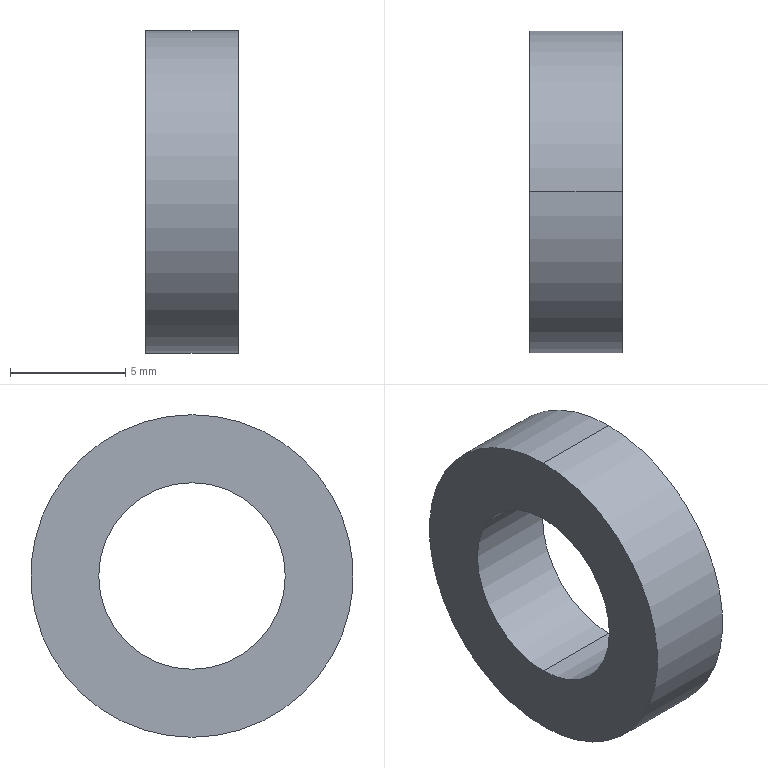Part | SolidWorks | features BaseBody 1 | 1 solid | 6 faces | box 4 x 14 x 14 mm | volume 409.632 mm3 | cylinder 4 | plane 2 | commonest cylinder face diameters 8.1 x2 14 x2
STEP:
#1=CARTESIAN_POINT('',(-2.,0.,-7.));
#2=VERTEX_POINT('',#1);
#3=CARTESIAN_POINT('',(-2.,0.,7.));
#4=VERTEX_POINT('',#3);
#5=CARTESIAN_POINT('',(-2.,0.,0.));
#6=DIRECTION('',(1.,0.,0.));
#7=DIRECTION('',(0.,0.,-1.));
#8=AXIS2_PLACEMENT_3D('',#5,#6,#7);
#9=CIRCLE('',#8,7.);
#10=EDGE_CURVE('',#2,#4,#9,.T.);
#11=ORIENTED_EDGE('',*,*,#10,.T.);
#12=CARTESIAN_POINT('',(2.,0.,7.));
#13=VERTEX_POINT('',#12);
#14=CARTESIAN_POINT('',(-2.,0.,7.));
#15=DIRECTION('',(1.,0.,0.));
#16=VECTOR('',#15,1000.);
#17=LINE('',#14,#16);
#18=EDGE_CURVE('',#4,#13,#17,.T.);
#19=ORIENTED_EDGE('',*,*,#18,.T.);
#20=CARTESIAN_POINT('',(2.,0.,-7.));
#21=VERTEX_POINT('',#20);
#22=CARTESIAN_POINT('',(2.,0.,0.));
#23=DIRECTION('',(-1.,0.,0.));
#24=DIRECTION('',(0.,0.,-1.));
#25=AXIS2_PLACEMENT_3D('',#22,#23,#24);
#26=CIRCLE('',#25,7.);
#27=EDGE_CURVE('',#13,#21,#26,.T.);
#28=ORIENTED_EDGE('',*,*,#27,.T.);
#29=CARTESIAN_POINT('',(-2.,0.,-7.));
#30=DIRECTION('',(1.,0.,0.));
#31=VECTOR('',#30,1000.);
#32=LINE('',#29,#31);
#33=EDGE_CURVE('',#2,#21,#32,.T.);
#34=ORIENTED_EDGE('',*,*,#33,.F.);
#35=EDGE_LOOP('',(#11,#19,#28,#34));
#36=FACE_OUTER_BOUND('',#35,.T.);
#37=CARTESIAN_POINT('',(-2.,0.,0.));
#38=DIRECTION('',(1.,0.,0.));
#39=DIRECTION('',(0.,0.,-1.));
#40=AXIS2_PLACEMENT_3D('',#37,#38,#39);
#41=CYLINDRICAL_SURFACE('',#40,7.);
#42=ADVANCED_FACE('',(#36),#41,.T.);
#43=CARTESIAN_POINT('',(-2.,0.,-4.05));
#44=VERTEX_POINT('',#43);
#45=CARTESIAN_POINT('',(-2.,0.,4.05));
#46=VERTEX_POINT('',#45);
#47=CARTESIAN_POINT('',(-2.,0.,0.));
#48=DIRECTION('',(-1.,0.,0.));
#49=DIRECTION('',(0.,0.,-1.));
#50=AXIS2_PLACEMENT_3D('',#47,#48,#49);
#51=CIRCLE('',#50,4.05);
#52=EDGE_CURVE('',#44,#46,#51,.T.);
#53=ORIENTED_EDGE('',*,*,#52,.T.);
#54=CARTESIAN_POINT('',(2.,0.,4.05));
#55=VERTEX_POINT('',#54);
#56=CARTESIAN_POINT('',(-3.,0.,4.05));
#57=DIRECTION('',(1.,0.,0.));
#58=VECTOR('',#57,1000.);
#59=LINE('',#56,#58);
#60=EDGE_CURVE('',#46,#55,#59,.T.);
#61=ORIENTED_EDGE('',*,*,#60,.T.);
#62=CARTESIAN_POINT('',(2.,0.,-4.05));
#63=VERTEX_POINT('',#62);
#64=CARTESIAN_POINT('',(2.,0.,0.));
#65=DIRECTION('',(-1.,0.,0.));
#66=DIRECTION('',(0.,0.,-1.));
#67=AXIS2_PLACEMENT_3D('',#64,#65,#66);
#68=CIRCLE('',#67,4.05);
#69=EDGE_CURVE('',#63,#55,#68,.T.);
#70=ORIENTED_EDGE('',*,*,#69,.F.);
#71=CARTESIAN_POINT('',(-3.,0.,-4.05));
#72=DIRECTION('',(1.,0.,0.));
#73=VECTOR('',#72,1000.);
#74=LINE('',#71,#73);
#75=EDGE_CURVE('',#44,#63,#74,.T.);
#76=ORIENTED_EDGE('',*,*,#75,.F.);
#77=EDGE_LOOP('',(#53,#61,#70,#76));
#78=FACE_OUTER_BOUND('',#77,.T.);
#79=CARTESIAN_POINT('',(-3.,0.,0.));
#80=DIRECTION('',(1.,0.,0.));
#81=DIRECTION('',(0.,0.,-1.));
#82=AXIS2_PLACEMENT_3D('',#79,#80,#81);
#83=CYLINDRICAL_SURFACE('',#82,4.05);
#84=ADVANCED_FACE('',(#78),#83,.F.);
#85=ORIENTED_EDGE('',*,*,#18,.F.);
#86=CARTESIAN_POINT('',(-2.,0.,0.));
#87=DIRECTION('',(1.,0.,0.));
#88=DIRECTION('',(0.,0.,-1.));
#89=AXIS2_PLACEMENT_3D('',#86,#87,#88);
#90=CIRCLE('',#89,7.);
#91=EDGE_CURVE('',#4,#2,#90,.T.);
#92=ORIENTED_EDGE('',*,*,#91,.T.);
#93=ORIENTED_EDGE('',*,*,#33,.T.);
#94=CARTESIAN_POINT('',(2.,0.,0.));
#95=DIRECTION('',(-1.,0.,0.));
#96=DIRECTION('',(0.,0.,-1.));
#97=AXIS2_PLACEMENT_3D('',#94,#95,#96);
#98=CIRCLE('',#97,7.);
#99=EDGE_CURVE('',#21,#13,#98,.T.);
#100=ORIENTED_EDGE('',*,*,#99,.T.);
#101=EDGE_LOOP('',(#85,#92,#93,#100));
#102=FACE_OUTER_BOUND('',#101,.T.);
#103=CARTESIAN_POINT('',(-2.,0.,0.));
#104=DIRECTION('',(1.,0.,0.));
#105=DIRECTION('',(0.,0.,-1.));
#106=AXIS2_PLACEMENT_3D('',#103,#104,#105);
#107=CYLINDRICAL_SURFACE('',#106,7.);
#108=ADVANCED_FACE('',(#102),#107,.T.);
#109=ORIENTED_EDGE('',*,*,#52,.F.);
#110=CARTESIAN_POINT('',(-2.,0.,0.));
#111=DIRECTION('',(-1.,0.,0.));
#112=DIRECTION('',(0.,0.,-1.));
#113=AXIS2_PLACEMENT_3D('',#110,#111,#112);
#114=CIRCLE('',#113,4.05);
#115=EDGE_CURVE('',#46,#44,#114,.T.);
#116=ORIENTED_EDGE('',*,*,#115,.F.);
#117=EDGE_LOOP('',(#109,#116));
#118=FACE_BOUND('',#117,.T.);
#119=ORIENTED_EDGE('',*,*,#10,.F.);
#120=ORIENTED_EDGE('',*,*,#91,.F.);
#121=EDGE_LOOP('',(#119,#120));
#122=FACE_OUTER_BOUND('',#121,.T.);
#123=CARTESIAN_POINT('',(-2.,0.,0.));
#124=DIRECTION('',(1.,0.,0.));
#125=DIRECTION('',(0.,0.,-1.));
#126=AXIS2_PLACEMENT_3D('',#123,#124,#125);
#127=PLANE('',#126);
#128=ADVANCED_FACE('',(#118,#122),#127,.F.);
#129=ORIENTED_EDGE('',*,*,#69,.T.);
#130=CARTESIAN_POINT('',(2.,0.,0.));
#131=DIRECTION('',(-1.,0.,0.));
#132=DIRECTION('',(0.,0.,-1.));
#133=AXIS2_PLACEMENT_3D('',#130,#131,#132);
#134=CIRCLE('',#133,4.05);
#135=EDGE_CURVE('',#55,#63,#134,.T.);
#136=ORIENTED_EDGE('',*,*,#135,.T.);
#137=EDGE_LOOP('',(#129,#136));
#138=FACE_BOUND('',#137,.T.);
#139=ORIENTED_EDGE('',*,*,#99,.F.);
#140=ORIENTED_EDGE('',*,*,#27,.F.);
#141=EDGE_LOOP('',(#139,#140));
#142=FACE_OUTER_BOUND('',#141,.T.);
#143=CARTESIAN_POINT('',(2.,0.,0.));
#144=DIRECTION('',(1.,0.,0.));
#145=DIRECTION('',(0.,0.,-1.));
#146=AXIS2_PLACEMENT_3D('',#143,#144,#145);
#147=PLANE('',#146);
#148=ADVANCED_FACE('',(#138,#142),#147,.T.);
#149=ORIENTED_EDGE('',*,*,#60,.F.);
#150=ORIENTED_EDGE('',*,*,#115,.T.);
#151=ORIENTED_EDGE('',*,*,#75,.T.);
#152=ORIENTED_EDGE('',*,*,#135,.F.);
#153=EDGE_LOOP('',(#149,#150,#151,#152));
#154=FACE_OUTER_BOUND('',#153,.T.);
#155=CARTESIAN_POINT('',(-3.,0.,0.));
#156=DIRECTION('',(1.,0.,0.));
#157=DIRECTION('',(0.,0.,-1.));
#158=AXIS2_PLACEMENT_3D('',#155,#156,#157);
#159=CYLINDRICAL_SURFACE('',#158,4.05);
#160=ADVANCED_FACE('',(#154),#159,.F.);
#161=CLOSED_SHELL('',(#42,#84,#108,#128,#148,#160));
#162=MANIFOLD_SOLID_BREP('',#161);
#163=CARTESIAN_POINT('',(0.,0.,0.));
#164=DIRECTION('',(0.,0.,1.));
#165=DIRECTION('',(1.,0.,0.));
#166=AXIS2_PLACEMENT_3D('',#163,#164,#165);
#167=(LENGTH_UNIT()NAMED_UNIT(*)SI_UNIT(.MILLI.,.METRE.));
#168=UNCERTAINTY_MEASURE_WITH_UNIT(LENGTH_MEASURE(0.00001),#167,'','');
#169=(NAMED_UNIT(*)PLANE_ANGLE_UNIT()SI_UNIT($,.RADIAN.));
#170=(NAMED_UNIT(*)SI_UNIT($,.STERADIAN.)SOLID_ANGLE_UNIT());
#171=(GEOMETRIC_REPRESENTATION_CONTEXT(3)GLOBAL_UNCERTAINTY_ASSIGNED_CONTEXT((#168))GLOBAL_UNIT_ASSIGNED_CONTEXT((#167,#169,#170))REPRESENTATION_CONTEXT('',''));
#172=ADVANCED_BREP_SHAPE_REPRESENTATION('',(#162,#166),#171);